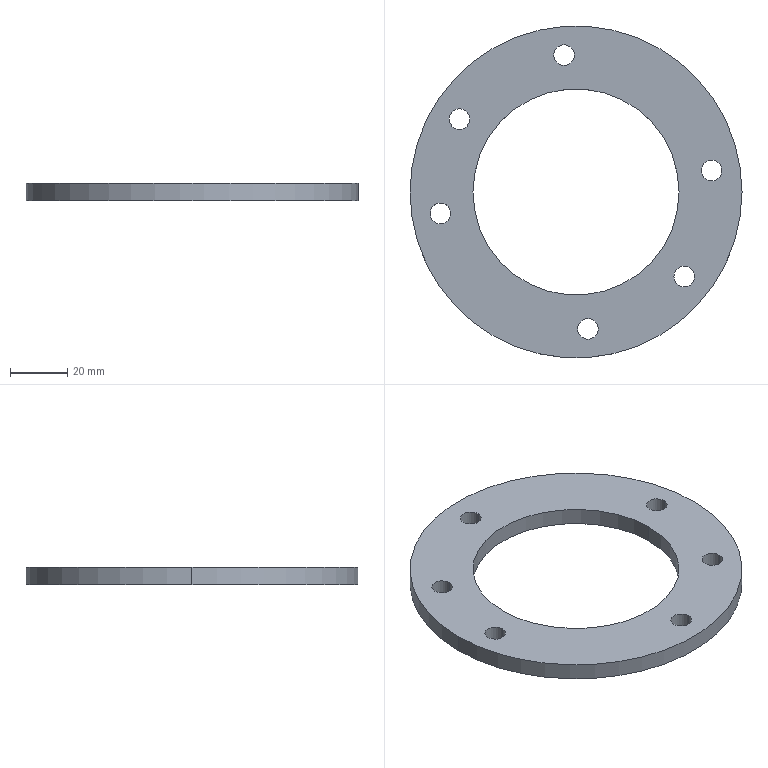Part | SolidWorks | features FlatPattern 1, SMBaseFlange 1, SheetMetal 1 | 1 solid | 18 faces | box 116 x 116 x 6 mm | volume 37515 mm3 | cylinder 16 | plane 2 | commonest cylinder face diameters 7.2 x12 72 x2 116 x2
STEP:
#1=CARTESIAN_POINT('',(-36.,0.,6.));
#2=VERTEX_POINT('',#1);
#3=CARTESIAN_POINT('',(36.,0.,6.));
#4=VERTEX_POINT('',#3);
#5=CARTESIAN_POINT('',(0.,0.,6.));
#6=DIRECTION('',(0.,0.,1.));
#7=DIRECTION('',(1.,0.,0.));
#8=AXIS2_PLACEMENT_3D('',#5,#6,#7);
#9=CIRCLE('',#8,36.);
#10=EDGE_CURVE('',#2,#4,#9,.T.);
#11=ORIENTED_EDGE('',*,*,#10,.T.);
#12=CARTESIAN_POINT('',(36.,0.,0.));
#13=VERTEX_POINT('',#12);
#14=CARTESIAN_POINT('',(36.,0.,6.));
#15=DIRECTION('',(0.,0.,-1.));
#16=VECTOR('',#15,1000.);
#17=LINE('',#14,#16);
#18=EDGE_CURVE('',#4,#13,#17,.T.);
#19=ORIENTED_EDGE('',*,*,#18,.T.);
#20=CARTESIAN_POINT('',(-36.,0.,0.));
#21=VERTEX_POINT('',#20);
#22=CARTESIAN_POINT('',(0.,0.,0.));
#23=DIRECTION('',(0.,0.,1.));
#24=DIRECTION('',(1.,0.,0.));
#25=AXIS2_PLACEMENT_3D('',#22,#23,#24);
#26=CIRCLE('',#25,36.);
#27=EDGE_CURVE('',#21,#13,#26,.T.);
#28=ORIENTED_EDGE('',*,*,#27,.F.);
#29=CARTESIAN_POINT('',(-36.,0.,6.));
#30=DIRECTION('',(0.,0.,-1.));
#31=VECTOR('',#30,1000.);
#32=LINE('',#29,#31);
#33=EDGE_CURVE('',#2,#21,#32,.T.);
#34=ORIENTED_EDGE('',*,*,#33,.F.);
#35=EDGE_LOOP('',(#11,#19,#28,#34));
#36=FACE_OUTER_BOUND('',#35,.T.);
#37=CARTESIAN_POINT('',(0.,0.,6.));
#38=DIRECTION('',(0.,0.,-1.));
#39=DIRECTION('',(-1.,0.,0.));
#40=AXIS2_PLACEMENT_3D('',#37,#38,#39);
#41=CYLINDRICAL_SURFACE('',#40,36.);
#42=ADVANCED_FACE('',(#36),#41,.F.);
#43=CARTESIAN_POINT('',(43.809,7.509,6.));
#44=VERTEX_POINT('',#43);
#45=CARTESIAN_POINT('',(51.009,7.509,6.));
#46=VERTEX_POINT('',#45);
#47=CARTESIAN_POINT('',(47.409,7.509,6.));
#48=DIRECTION('',(0.,0.,1.));
#49=DIRECTION('',(1.,0.,0.));
#50=AXIS2_PLACEMENT_3D('',#47,#48,#49);
#51=CIRCLE('',#50,3.6);
#52=EDGE_CURVE('',#44,#46,#51,.T.);
#53=ORIENTED_EDGE('',*,*,#52,.T.);
#54=CARTESIAN_POINT('',(51.009,7.509,0.));
#55=VERTEX_POINT('',#54);
#56=CARTESIAN_POINT('',(51.009,7.509,6.));
#57=DIRECTION('',(0.,0.,-1.));
#58=VECTOR('',#57,1000.);
#59=LINE('',#56,#58);
#60=EDGE_CURVE('',#46,#55,#59,.T.);
#61=ORIENTED_EDGE('',*,*,#60,.T.);
#62=CARTESIAN_POINT('',(43.809,7.509,0.));
#63=VERTEX_POINT('',#62);
#64=CARTESIAN_POINT('',(47.409,7.509,0.));
#65=DIRECTION('',(0.,0.,1.));
#66=DIRECTION('',(1.,0.,0.));
#67=AXIS2_PLACEMENT_3D('',#64,#65,#66);
#68=CIRCLE('',#67,3.6);
#69=EDGE_CURVE('',#63,#55,#68,.T.);
#70=ORIENTED_EDGE('',*,*,#69,.F.);
#71=CARTESIAN_POINT('',(43.809,7.509,6.));
#72=DIRECTION('',(0.,0.,-1.));
#73=VECTOR('',#72,1000.);
#74=LINE('',#71,#73);
#75=EDGE_CURVE('',#44,#63,#74,.T.);
#76=ORIENTED_EDGE('',*,*,#75,.F.);
#77=EDGE_LOOP('',(#53,#61,#70,#76));
#78=FACE_OUTER_BOUND('',#77,.T.);
#79=CARTESIAN_POINT('',(47.409,7.509,6.));
#80=DIRECTION('',(0.,0.,-1.));
#81=DIRECTION('',(-1.,0.,0.));
#82=AXIS2_PLACEMENT_3D('',#79,#80,#81);
#83=CYLINDRICAL_SURFACE('',#82,3.6);
#84=ADVANCED_FACE('',(#78),#83,.F.);
#85=CARTESIAN_POINT('',(34.225,-29.552,6.));
#86=VERTEX_POINT('',#85);
#87=CARTESIAN_POINT('',(41.425,-29.552,6.));
#88=VERTEX_POINT('',#87);
#89=CARTESIAN_POINT('',(37.825,-29.552,6.));
#90=DIRECTION('',(0.,0.,1.));
#91=DIRECTION('',(1.,0.,0.));
#92=AXIS2_PLACEMENT_3D('',#89,#90,#91);
#93=CIRCLE('',#92,3.6);
#94=EDGE_CURVE('',#86,#88,#93,.T.);
#95=ORIENTED_EDGE('',*,*,#94,.T.);
#96=CARTESIAN_POINT('',(41.425,-29.552,0.));
#97=VERTEX_POINT('',#96);
#98=CARTESIAN_POINT('',(41.425,-29.552,6.));
#99=DIRECTION('',(0.,0.,-1.));
#100=VECTOR('',#99,1000.);
#101=LINE('',#98,#100);
#102=EDGE_CURVE('',#88,#97,#101,.T.);
#103=ORIENTED_EDGE('',*,*,#102,.T.);
#104=CARTESIAN_POINT('',(34.225,-29.552,0.));
#105=VERTEX_POINT('',#104);
#106=CARTESIAN_POINT('',(37.825,-29.552,0.));
#107=DIRECTION('',(0.,0.,1.));
#108=DIRECTION('',(1.,0.,0.));
#109=AXIS2_PLACEMENT_3D('',#106,#107,#108);
#110=CIRCLE('',#109,3.6);
#111=EDGE_CURVE('',#105,#97,#110,.T.);
#112=ORIENTED_EDGE('',*,*,#111,.F.);
#113=CARTESIAN_POINT('',(34.225,-29.552,6.));
#114=DIRECTION('',(0.,0.,-1.));
#115=VECTOR('',#114,1000.);
#116=LINE('',#113,#115);
#117=EDGE_CURVE('',#86,#105,#116,.T.);
#118=ORIENTED_EDGE('',*,*,#117,.F.);
#119=EDGE_LOOP('',(#95,#103,#112,#118));
#120=FACE_OUTER_BOUND('',#119,.T.);
#121=CARTESIAN_POINT('',(37.825,-29.552,6.));
#122=DIRECTION('',(0.,0.,-1.));
#123=DIRECTION('',(-1.,0.,0.));
#124=AXIS2_PLACEMENT_3D('',#121,#122,#123);
#125=CYLINDRICAL_SURFACE('',#124,3.6);
#126=ADVANCED_FACE('',(#120),#125,.F.);
#127=CARTESIAN_POINT('',(0.5835,-47.817,6.));
#128=VERTEX_POINT('',#127);
#129=CARTESIAN_POINT('',(7.783,-47.817,6.));
#130=VERTEX_POINT('',#129);
#131=CARTESIAN_POINT('',(4.183,-47.817,6.));
#132=DIRECTION('',(0.,0.,1.));
#133=DIRECTION('',(1.,0.,0.));
#134=AXIS2_PLACEMENT_3D('',#131,#132,#133);
#135=CIRCLE('',#134,3.6);
#136=EDGE_CURVE('',#128,#130,#135,.T.);
#137=ORIENTED_EDGE('',*,*,#136,.T.);
#138=CARTESIAN_POINT('',(7.783,-47.817,0.));
#139=VERTEX_POINT('',#138);
#140=CARTESIAN_POINT('',(7.783,-47.817,6.));
#141=DIRECTION('',(0.,0.,-1.));
#142=VECTOR('',#141,1000.);
#143=LINE('',#140,#142);
#144=EDGE_CURVE('',#130,#139,#143,.T.);
#145=ORIENTED_EDGE('',*,*,#144,.T.);
#146=CARTESIAN_POINT('',(0.5835,-47.817,0.));
#147=VERTEX_POINT('',#146);
#148=CARTESIAN_POINT('',(4.183,-47.817,0.));
#149=DIRECTION('',(0.,0.,1.));
#150=DIRECTION('',(1.,0.,0.));
#151=AXIS2_PLACEMENT_3D('',#148,#149,#150);
#152=CIRCLE('',#151,3.6);
#153=EDGE_CURVE('',#147,#139,#152,.T.);
#154=ORIENTED_EDGE('',*,*,#153,.F.);
#155=CARTESIAN_POINT('',(0.5835,-47.817,6.));
#156=DIRECTION('',(0.,0.,-1.));
#157=VECTOR('',#156,1000.);
#158=LINE('',#155,#157);
#159=EDGE_CURVE('',#128,#147,#158,.T.);
#160=ORIENTED_EDGE('',*,*,#159,.F.);
#161=EDGE_LOOP('',(#137,#145,#154,#160));
#162=FACE_OUTER_BOUND('',#161,.T.);
#163=CARTESIAN_POINT('',(4.183,-47.817,6.));
#164=DIRECTION('',(0.,0.,-1.));
#165=DIRECTION('',(-1.,0.,0.));
#166=AXIS2_PLACEMENT_3D('',#163,#164,#165);
#167=CYLINDRICAL_SURFACE('',#166,3.6);
#168=ADVANCED_FACE('',(#162),#167,.F.);
#169=CARTESIAN_POINT('',(-51.009,-7.509,6.));
#170=VERTEX_POINT('',#169);
#171=CARTESIAN_POINT('',(-43.809,-7.509,6.));
#172=VERTEX_POINT('',#171);
#173=CARTESIAN_POINT('',(-47.409,-7.509,6.));
#174=DIRECTION('',(0.,0.,1.));
#175=DIRECTION('',(1.,0.,0.));
#176=AXIS2_PLACEMENT_3D('',#173,#174,#175);
#177=CIRCLE('',#176,3.6);
#178=EDGE_CURVE('',#170,#172,#177,.T.);
#179=ORIENTED_EDGE('',*,*,#178,.T.);
#180=CARTESIAN_POINT('',(-43.809,-7.509,0.));
#181=VERTEX_POINT('',#180);
#182=CARTESIAN_POINT('',(-43.809,-7.509,6.));
#183=DIRECTION('',(0.,0.,-1.));
#184=VECTOR('',#183,1000.);
#185=LINE('',#182,#184);
#186=EDGE_CURVE('',#172,#181,#185,.T.);
#187=ORIENTED_EDGE('',*,*,#186,.T.);
#188=CARTESIAN_POINT('',(-51.009,-7.509,0.));
#189=VERTEX_POINT('',#188);
#190=CARTESIAN_POINT('',(-47.409,-7.509,0.));
#191=DIRECTION('',(0.,0.,1.));
#192=DIRECTION('',(1.,0.,0.));
#193=AXIS2_PLACEMENT_3D('',#190,#191,#192);
#194=CIRCLE('',#193,3.6);
#195=EDGE_CURVE('',#189,#181,#194,.T.);
#196=ORIENTED_EDGE('',*,*,#195,.F.);
#197=CARTESIAN_POINT('',(-51.009,-7.509,6.));
#198=DIRECTION('',(0.,0.,-1.));
#199=VECTOR('',#198,1000.);
#200=LINE('',#197,#199);
#201=EDGE_CURVE('',#170,#189,#200,.T.);
#202=ORIENTED_EDGE('',*,*,#201,.F.);
#203=EDGE_LOOP('',(#179,#187,#196,#202));
#204=FACE_OUTER_BOUND('',#203,.T.);
#205=CARTESIAN_POINT('',(-47.409,-7.509,6.));
#206=DIRECTION('',(0.,0.,-1.));
#207=DIRECTION('',(-1.,0.,0.));
#208=AXIS2_PLACEMENT_3D('',#205,#206,#207);
#209=CYLINDRICAL_SURFACE('',#208,3.6);
#210=ADVANCED_FACE('',(#204),#209,.F.);
#211=CARTESIAN_POINT('',(-44.306,25.436,6.));
#212=VERTEX_POINT('',#211);
#213=CARTESIAN_POINT('',(-37.106,25.436,6.));
#214=VERTEX_POINT('',#213);
#215=CARTESIAN_POINT('',(-40.706,25.436,6.));
#216=DIRECTION('',(0.,0.,1.));
#217=DIRECTION('',(1.,0.,0.));
#218=AXIS2_PLACEMENT_3D('',#215,#216,#217);
#219=CIRCLE('',#218,3.6);
#220=EDGE_CURVE('',#212,#214,#219,.T.);
#221=ORIENTED_EDGE('',*,*,#220,.T.);
#222=CARTESIAN_POINT('',(-37.106,25.436,0.));
#223=VERTEX_POINT('',#222);
#224=CARTESIAN_POINT('',(-37.106,25.436,6.));
#225=DIRECTION('',(0.,0.,-1.));
#226=VECTOR('',#225,1000.);
#227=LINE('',#224,#226);
#228=EDGE_CURVE('',#214,#223,#227,.T.);
#229=ORIENTED_EDGE('',*,*,#228,.T.);
#230=CARTESIAN_POINT('',(-44.306,25.436,0.));
#231=VERTEX_POINT('',#230);
#232=CARTESIAN_POINT('',(-40.706,25.436,0.));
#233=DIRECTION('',(0.,0.,1.));
#234=DIRECTION('',(1.,0.,0.));
#235=AXIS2_PLACEMENT_3D('',#232,#233,#234);
#236=CIRCLE('',#235,3.6);
#237=EDGE_CURVE('',#231,#223,#236,.T.);
#238=ORIENTED_EDGE('',*,*,#237,.F.);
#239=CARTESIAN_POINT('',(-44.306,25.436,6.));
#240=DIRECTION('',(0.,0.,-1.));
#241=VECTOR('',#240,1000.);
#242=LINE('',#239,#241);
#243=EDGE_CURVE('',#212,#231,#242,.T.);
#244=ORIENTED_EDGE('',*,*,#243,.F.);
#245=EDGE_LOOP('',(#221,#229,#238,#244));
#246=FACE_OUTER_BOUND('',#245,.T.);
#247=CARTESIAN_POINT('',(-40.706,25.436,6.));
#248=DIRECTION('',(0.,0.,-1.));
#249=DIRECTION('',(-1.,0.,0.));
#250=AXIS2_PLACEMENT_3D('',#247,#248,#249);
#251=CYLINDRICAL_SURFACE('',#250,3.6);
#252=ADVANCED_FACE('',(#246),#251,.F.);
#253=CARTESIAN_POINT('',(-7.783,47.817,6.));
#254=VERTEX_POINT('',#253);
#255=CARTESIAN_POINT('',(-0.5835,47.817,6.));
#256=VERTEX_POINT('',#255);
#257=CARTESIAN_POINT('',(-4.183,47.817,6.));
#258=DIRECTION('',(0.,0.,1.));
#259=DIRECTION('',(1.,0.,0.));
#260=AXIS2_PLACEMENT_3D('',#257,#258,#259);
#261=CIRCLE('',#260,3.6);
#262=EDGE_CURVE('',#254,#256,#261,.T.);
#263=ORIENTED_EDGE('',*,*,#262,.T.);
#264=CARTESIAN_POINT('',(-0.5835,47.817,0.));
#265=VERTEX_POINT('',#264);
#266=CARTESIAN_POINT('',(-0.5835,47.817,6.));
#267=DIRECTION('',(0.,0.,-1.));
#268=VECTOR('',#267,1000.);
#269=LINE('',#266,#268);
#270=EDGE_CURVE('',#256,#265,#269,.T.);
#271=ORIENTED_EDGE('',*,*,#270,.T.);
#272=CARTESIAN_POINT('',(-7.783,47.817,0.));
#273=VERTEX_POINT('',#272);
#274=CARTESIAN_POINT('',(-4.183,47.817,0.));
#275=DIRECTION('',(0.,0.,1.));
#276=DIRECTION('',(1.,0.,0.));
#277=AXIS2_PLACEMENT_3D('',#274,#275,#276);
#278=CIRCLE('',#277,3.6);
#279=EDGE_CURVE('',#273,#265,#278,.T.);
#280=ORIENTED_EDGE('',*,*,#279,.F.);
#281=CARTESIAN_POINT('',(-7.783,47.817,6.));
#282=DIRECTION('',(0.,0.,-1.));
#283=VECTOR('',#282,1000.);
#284=LINE('',#281,#283);
#285=EDGE_CURVE('',#254,#273,#284,.T.);
#286=ORIENTED_EDGE('',*,*,#285,.F.);
#287=EDGE_LOOP('',(#263,#271,#280,#286));
#288=FACE_OUTER_BOUND('',#287,.T.);
#289=CARTESIAN_POINT('',(-4.183,47.817,6.));
#290=DIRECTION('',(0.,0.,-1.));
#291=DIRECTION('',(-1.,0.,0.));
#292=AXIS2_PLACEMENT_3D('',#289,#290,#291);
#293=CYLINDRICAL_SURFACE('',#292,3.6);
#294=ADVANCED_FACE('',(#288),#293,.F.);
#295=CARTESIAN_POINT('',(58.,0.,6.));
#296=VERTEX_POINT('',#295);
#297=CARTESIAN_POINT('',(-58.,0.,6.));
#298=VERTEX_POINT('',#297);
#299=CARTESIAN_POINT('',(0.,0.,6.));
#300=DIRECTION('',(0.,0.,1.));
#301=DIRECTION('',(1.,0.,0.));
#302=AXIS2_PLACEMENT_3D('',#299,#300,#301);
#303=CIRCLE('',#302,58.);
#304=EDGE_CURVE('',#296,#298,#303,.T.);
#305=ORIENTED_EDGE('',*,*,#304,.F.);
#306=CARTESIAN_POINT('',(58.,0.,0.));
#307=VERTEX_POINT('',#306);
#308=CARTESIAN_POINT('',(58.,0.,6.));
#309=DIRECTION('',(0.,0.,-1.));
#310=VECTOR('',#309,1000.);
#311=LINE('',#308,#310);
#312=EDGE_CURVE('',#296,#307,#311,.T.);
#313=ORIENTED_EDGE('',*,*,#312,.T.);
#314=CARTESIAN_POINT('',(-58.,0.,0.));
#315=VERTEX_POINT('',#314);
#316=CARTESIAN_POINT('',(0.,0.,0.));
#317=DIRECTION('',(0.,0.,1.));
#318=DIRECTION('',(1.,0.,0.));
#319=AXIS2_PLACEMENT_3D('',#316,#317,#318);
#320=CIRCLE('',#319,58.);
#321=EDGE_CURVE('',#307,#315,#320,.T.);
#322=ORIENTED_EDGE('',*,*,#321,.T.);
#323=CARTESIAN_POINT('',(-58.,0.,6.));
#324=DIRECTION('',(0.,0.,-1.));
#325=VECTOR('',#324,1000.);
#326=LINE('',#323,#325);
#327=EDGE_CURVE('',#298,#315,#326,.T.);
#328=ORIENTED_EDGE('',*,*,#327,.F.);
#329=EDGE_LOOP('',(#305,#313,#322,#328));
#330=FACE_OUTER_BOUND('',#329,.T.);
#331=CARTESIAN_POINT('',(0.,0.,6.));
#332=DIRECTION('',(0.,0.,-1.));
#333=DIRECTION('',(-1.,0.,0.));
#334=AXIS2_PLACEMENT_3D('',#331,#332,#333);
#335=CYLINDRICAL_SURFACE('',#334,58.);
#336=ADVANCED_FACE('',(#330),#335,.T.);
#337=ORIENTED_EDGE('',*,*,#52,.F.);
#338=CARTESIAN_POINT('',(47.409,7.509,6.));
#339=DIRECTION('',(0.,0.,1.));
#340=DIRECTION('',(1.,0.,0.));
#341=AXIS2_PLACEMENT_3D('',#338,#339,#340);
#342=CIRCLE('',#341,3.6);
#343=EDGE_CURVE('',#46,#44,#342,.T.);
#344=ORIENTED_EDGE('',*,*,#343,.F.);
#345=EDGE_LOOP('',(#337,#344));
#346=FACE_BOUND('',#345,.T.);
#347=ORIENTED_EDGE('',*,*,#136,.F.);
#348=CARTESIAN_POINT('',(4.183,-47.817,6.));
#349=DIRECTION('',(0.,0.,1.));
#350=DIRECTION('',(1.,0.,0.));
#351=AXIS2_PLACEMENT_3D('',#348,#349,#350);
#352=CIRCLE('',#351,3.6);
#353=EDGE_CURVE('',#130,#128,#352,.T.);
#354=ORIENTED_EDGE('',*,*,#353,.F.);
#355=EDGE_LOOP('',(#347,#354));
#356=FACE_BOUND('',#355,.T.);
#357=ORIENTED_EDGE('',*,*,#220,.F.);
#358=CARTESIAN_POINT('',(-40.706,25.436,6.));
#359=DIRECTION('',(0.,0.,1.));
#360=DIRECTION('',(1.,0.,0.));
#361=AXIS2_PLACEMENT_3D('',#358,#359,#360);
#362=CIRCLE('',#361,3.6);
#363=EDGE_CURVE('',#214,#212,#362,.T.);
#364=ORIENTED_EDGE('',*,*,#363,.F.);
#365=EDGE_LOOP('',(#357,#364));
#366=FACE_BOUND('',#365,.T.);
#367=CARTESIAN_POINT('',(0.,0.,6.));
#368=DIRECTION('',(0.,0.,1.));
#369=DIRECTION('',(1.,0.,0.));
#370=AXIS2_PLACEMENT_3D('',#367,#368,#369);
#371=CIRCLE('',#370,58.);
#372=EDGE_CURVE('',#298,#296,#371,.T.);
#373=ORIENTED_EDGE('',*,*,#372,.T.);
#374=ORIENTED_EDGE('',*,*,#304,.T.);
#375=EDGE_LOOP('',(#373,#374));
#376=FACE_OUTER_BOUND('',#375,.T.);
#377=ORIENTED_EDGE('',*,*,#262,.F.);
#378=CARTESIAN_POINT('',(-4.183,47.817,6.));
#379=DIRECTION('',(0.,0.,1.));
#380=DIRECTION('',(1.,0.,0.));
#381=AXIS2_PLACEMENT_3D('',#378,#379,#380);
#382=CIRCLE('',#381,3.6);
#383=EDGE_CURVE('',#256,#254,#382,.T.);
#384=ORIENTED_EDGE('',*,*,#383,.F.);
#385=EDGE_LOOP('',(#377,#384));
#386=FACE_BOUND('',#385,.T.);
#387=ORIENTED_EDGE('',*,*,#178,.F.);
#388=CARTESIAN_POINT('',(-47.409,-7.509,6.));
#389=DIRECTION('',(0.,0.,1.));
#390=DIRECTION('',(1.,0.,0.));
#391=AXIS2_PLACEMENT_3D('',#388,#389,#390);
#392=CIRCLE('',#391,3.6);
#393=EDGE_CURVE('',#172,#170,#392,.T.);
#394=ORIENTED_EDGE('',*,*,#393,.F.);
#395=EDGE_LOOP('',(#387,#394));
#396=FACE_BOUND('',#395,.T.);
#397=ORIENTED_EDGE('',*,*,#94,.F.);
#398=CARTESIAN_POINT('',(37.825,-29.552,6.));
#399=DIRECTION('',(0.,0.,1.));
#400=DIRECTION('',(1.,0.,0.));
#401=AXIS2_PLACEMENT_3D('',#398,#399,#400);
#402=CIRCLE('',#401,3.6);
#403=EDGE_CURVE('',#88,#86,#402,.T.);
#404=ORIENTED_EDGE('',*,*,#403,.F.);
#405=EDGE_LOOP('',(#397,#404));
#406=FACE_BOUND('',#405,.T.);
#407=ORIENTED_EDGE('',*,*,#10,.F.);
#408=CARTESIAN_POINT('',(0.,0.,6.));
#409=DIRECTION('',(0.,0.,1.));
#410=DIRECTION('',(1.,0.,0.));
#411=AXIS2_PLACEMENT_3D('',#408,#409,#410);
#412=CIRCLE('',#411,36.);
#413=EDGE_CURVE('',#4,#2,#412,.T.);
#414=ORIENTED_EDGE('',*,*,#413,.F.);
#415=EDGE_LOOP('',(#407,#414));
#416=FACE_BOUND('',#415,.T.);
#417=CARTESIAN_POINT('',(0.,0.,6.));
#418=DIRECTION('',(0.,0.,1.));
#419=DIRECTION('',(1.,0.,0.));
#420=AXIS2_PLACEMENT_3D('',#417,#418,#419);
#421=PLANE('',#420);
#422=ADVANCED_FACE('',(#346,#356,#366,#376,#386,#396,#406,#416),#421,.T.);
#423=CARTESIAN_POINT('',(0.,0.,0.));
#424=DIRECTION('',(0.,0.,1.));
#425=DIRECTION('',(1.,0.,0.));
#426=AXIS2_PLACEMENT_3D('',#423,#424,#425);
#427=CIRCLE('',#426,58.);
#428=EDGE_CURVE('',#315,#307,#427,.T.);
#429=ORIENTED_EDGE('',*,*,#428,.F.);
#430=ORIENTED_EDGE('',*,*,#321,.F.);
#431=EDGE_LOOP('',(#429,#430));
#432=FACE_OUTER_BOUND('',#431,.T.);
#433=ORIENTED_EDGE('',*,*,#279,.T.);
#434=CARTESIAN_POINT('',(-4.183,47.817,0.));
#435=DIRECTION('',(0.,0.,1.));
#436=DIRECTION('',(1.,0.,0.));
#437=AXIS2_PLACEMENT_3D('',#434,#435,#436);
#438=CIRCLE('',#437,3.6);
#439=EDGE_CURVE('',#265,#273,#438,.T.);
#440=ORIENTED_EDGE('',*,*,#439,.T.);
#441=EDGE_LOOP('',(#433,#440));
#442=FACE_BOUND('',#441,.T.);
#443=ORIENTED_EDGE('',*,*,#237,.T.);
#444=CARTESIAN_POINT('',(-40.706,25.436,0.));
#445=DIRECTION('',(0.,0.,1.));
#446=DIRECTION('',(1.,0.,0.));
#447=AXIS2_PLACEMENT_3D('',#444,#445,#446);
#448=CIRCLE('',#447,3.6);
#449=EDGE_CURVE('',#223,#231,#448,.T.);
#450=ORIENTED_EDGE('',*,*,#449,.T.);
#451=EDGE_LOOP('',(#443,#450));
#452=FACE_BOUND('',#451,.T.);
#453=ORIENTED_EDGE('',*,*,#195,.T.);
#454=CARTESIAN_POINT('',(-47.409,-7.509,0.));
#455=DIRECTION('',(0.,0.,1.));
#456=DIRECTION('',(1.,0.,0.));
#457=AXIS2_PLACEMENT_3D('',#454,#455,#456);
#458=CIRCLE('',#457,3.6);
#459=EDGE_CURVE('',#181,#189,#458,.T.);
#460=ORIENTED_EDGE('',*,*,#459,.T.);
#461=EDGE_LOOP('',(#453,#460));
#462=FACE_BOUND('',#461,.T.);
#463=ORIENTED_EDGE('',*,*,#153,.T.);
#464=CARTESIAN_POINT('',(4.183,-47.817,0.));
#465=DIRECTION('',(0.,0.,1.));
#466=DIRECTION('',(1.,0.,0.));
#467=AXIS2_PLACEMENT_3D('',#464,#465,#466);
#468=CIRCLE('',#467,3.6);
#469=EDGE_CURVE('',#139,#147,#468,.T.);
#470=ORIENTED_EDGE('',*,*,#469,.T.);
#471=EDGE_LOOP('',(#463,#470));
#472=FACE_BOUND('',#471,.T.);
#473=ORIENTED_EDGE('',*,*,#111,.T.);
#474=CARTESIAN_POINT('',(37.825,-29.552,0.));
#475=DIRECTION('',(0.,0.,1.));
#476=DIRECTION('',(1.,0.,0.));
#477=AXIS2_PLACEMENT_3D('',#474,#475,#476);
#478=CIRCLE('',#477,3.6);
#479=EDGE_CURVE('',#97,#105,#478,.T.);
#480=ORIENTED_EDGE('',*,*,#479,.T.);
#481=EDGE_LOOP('',(#473,#480));
#482=FACE_BOUND('',#481,.T.);
#483=ORIENTED_EDGE('',*,*,#69,.T.);
#484=CARTESIAN_POINT('',(47.409,7.509,0.));
#485=DIRECTION('',(0.,0.,1.));
#486=DIRECTION('',(1.,0.,0.));
#487=AXIS2_PLACEMENT_3D('',#484,#485,#486);
#488=CIRCLE('',#487,3.6);
#489=EDGE_CURVE('',#55,#63,#488,.T.);
#490=ORIENTED_EDGE('',*,*,#489,.T.);
#491=EDGE_LOOP('',(#483,#490));
#492=FACE_BOUND('',#491,.T.);
#493=ORIENTED_EDGE('',*,*,#27,.T.);
#494=CARTESIAN_POINT('',(0.,0.,0.));
#495=DIRECTION('',(0.,0.,1.));
#496=DIRECTION('',(1.,0.,0.));
#497=AXIS2_PLACEMENT_3D('',#494,#495,#496);
#498=CIRCLE('',#497,36.);
#499=EDGE_CURVE('',#13,#21,#498,.T.);
#500=ORIENTED_EDGE('',*,*,#499,.T.);
#501=EDGE_LOOP('',(#493,#500));
#502=FACE_BOUND('',#501,.T.);
#503=CARTESIAN_POINT('',(0.,0.,0.));
#504=DIRECTION('',(0.,0.,1.));
#505=DIRECTION('',(1.,0.,0.));
#506=AXIS2_PLACEMENT_3D('',#503,#504,#505);
#507=PLANE('',#506);
#508=ADVANCED_FACE('',(#432,#442,#452,#462,#472,#482,#492,#502),#507,.F.);
#509=ORIENTED_EDGE('',*,*,#312,.F.);
#510=ORIENTED_EDGE('',*,*,#372,.F.);
#511=ORIENTED_EDGE('',*,*,#327,.T.);
#512=ORIENTED_EDGE('',*,*,#428,.T.);
#513=EDGE_LOOP('',(#509,#510,#511,#512));
#514=FACE_OUTER_BOUND('',#513,.T.);
#515=CARTESIAN_POINT('',(0.,0.,6.));
#516=DIRECTION('',(0.,0.,-1.));
#517=DIRECTION('',(-1.,0.,0.));
#518=AXIS2_PLACEMENT_3D('',#515,#516,#517);
#519=CYLINDRICAL_SURFACE('',#518,58.);
#520=ADVANCED_FACE('',(#514),#519,.T.);
#521=ORIENTED_EDGE('',*,*,#270,.F.);
#522=ORIENTED_EDGE('',*,*,#383,.T.);
#523=ORIENTED_EDGE('',*,*,#285,.T.);
#524=ORIENTED_EDGE('',*,*,#439,.F.);
#525=EDGE_LOOP('',(#521,#522,#523,#524));
#526=FACE_OUTER_BOUND('',#525,.T.);
#527=CARTESIAN_POINT('',(-4.183,47.817,6.));
#528=DIRECTION('',(0.,0.,-1.));
#529=DIRECTION('',(-1.,0.,0.));
#530=AXIS2_PLACEMENT_3D('',#527,#528,#529);
#531=CYLINDRICAL_SURFACE('',#530,3.6);
#532=ADVANCED_FACE('',(#526),#531,.F.);
#533=ORIENTED_EDGE('',*,*,#228,.F.);
#534=ORIENTED_EDGE('',*,*,#363,.T.);
#535=ORIENTED_EDGE('',*,*,#243,.T.);
#536=ORIENTED_EDGE('',*,*,#449,.F.);
#537=EDGE_LOOP('',(#533,#534,#535,#536));
#538=FACE_OUTER_BOUND('',#537,.T.);
#539=CARTESIAN_POINT('',(-40.706,25.436,6.));
#540=DIRECTION('',(0.,0.,-1.));
#541=DIRECTION('',(-1.,0.,0.));
#542=AXIS2_PLACEMENT_3D('',#539,#540,#541);
#543=CYLINDRICAL_SURFACE('',#542,3.6);
#544=ADVANCED_FACE('',(#538),#543,.F.);
#545=ORIENTED_EDGE('',*,*,#186,.F.);
#546=ORIENTED_EDGE('',*,*,#393,.T.);
#547=ORIENTED_EDGE('',*,*,#201,.T.);
#548=ORIENTED_EDGE('',*,*,#459,.F.);
#549=EDGE_LOOP('',(#545,#546,#547,#548));
#550=FACE_OUTER_BOUND('',#549,.T.);
#551=CARTESIAN_POINT('',(-47.409,-7.509,6.));
#552=DIRECTION('',(0.,0.,-1.));
#553=DIRECTION('',(-1.,0.,0.));
#554=AXIS2_PLACEMENT_3D('',#551,#552,#553);
#555=CYLINDRICAL_SURFACE('',#554,3.6);
#556=ADVANCED_FACE('',(#550),#555,.F.);
#557=ORIENTED_EDGE('',*,*,#144,.F.);
#558=ORIENTED_EDGE('',*,*,#353,.T.);
#559=ORIENTED_EDGE('',*,*,#159,.T.);
#560=ORIENTED_EDGE('',*,*,#469,.F.);
#561=EDGE_LOOP('',(#557,#558,#559,#560));
#562=FACE_OUTER_BOUND('',#561,.T.);
#563=CARTESIAN_POINT('',(4.183,-47.817,6.));
#564=DIRECTION('',(0.,0.,-1.));
#565=DIRECTION('',(-1.,0.,0.));
#566=AXIS2_PLACEMENT_3D('',#563,#564,#565);
#567=CYLINDRICAL_SURFACE('',#566,3.6);
#568=ADVANCED_FACE('',(#562),#567,.F.);
#569=ORIENTED_EDGE('',*,*,#102,.F.);
#570=ORIENTED_EDGE('',*,*,#403,.T.);
#571=ORIENTED_EDGE('',*,*,#117,.T.);
#572=ORIENTED_EDGE('',*,*,#479,.F.);
#573=EDGE_LOOP('',(#569,#570,#571,#572));
#574=FACE_OUTER_BOUND('',#573,.T.);
#575=CARTESIAN_POINT('',(37.825,-29.552,6.));
#576=DIRECTION('',(0.,0.,-1.));
#577=DIRECTION('',(-1.,0.,0.));
#578=AXIS2_PLACEMENT_3D('',#575,#576,#577);
#579=CYLINDRICAL_SURFACE('',#578,3.6);
#580=ADVANCED_FACE('',(#574),#579,.F.);
#581=ORIENTED_EDGE('',*,*,#60,.F.);
#582=ORIENTED_EDGE('',*,*,#343,.T.);
#583=ORIENTED_EDGE('',*,*,#75,.T.);
#584=ORIENTED_EDGE('',*,*,#489,.F.);
#585=EDGE_LOOP('',(#581,#582,#583,#584));
#586=FACE_OUTER_BOUND('',#585,.T.);
#587=CARTESIAN_POINT('',(47.409,7.509,6.));
#588=DIRECTION('',(0.,0.,-1.));
#589=DIRECTION('',(-1.,0.,0.));
#590=AXIS2_PLACEMENT_3D('',#587,#588,#589);
#591=CYLINDRICAL_SURFACE('',#590,3.6);
#592=ADVANCED_FACE('',(#586),#591,.F.);
#593=ORIENTED_EDGE('',*,*,#18,.F.);
#594=ORIENTED_EDGE('',*,*,#413,.T.);
#595=ORIENTED_EDGE('',*,*,#33,.T.);
#596=ORIENTED_EDGE('',*,*,#499,.F.);
#597=EDGE_LOOP('',(#593,#594,#595,#596));
#598=FACE_OUTER_BOUND('',#597,.T.);
#599=CARTESIAN_POINT('',(0.,0.,6.));
#600=DIRECTION('',(0.,0.,-1.));
#601=DIRECTION('',(-1.,0.,0.));
#602=AXIS2_PLACEMENT_3D('',#599,#600,#601);
#603=CYLINDRICAL_SURFACE('',#602,36.);
#604=ADVANCED_FACE('',(#598),#603,.F.);
#605=CLOSED_SHELL('',(#42,#84,#126,#168,#210,#252,#294,#336,#422,#508,#520,#532,#544,#556,#568,#580,#592,#604));
#606=MANIFOLD_SOLID_BREP('',#605);
#607=CARTESIAN_POINT('',(0.,0.,0.));
#608=DIRECTION('',(0.,0.,1.));
#609=DIRECTION('',(1.,0.,0.));
#610=AXIS2_PLACEMENT_3D('',#607,#608,#609);
#611=(LENGTH_UNIT()NAMED_UNIT(*)SI_UNIT(.MILLI.,.METRE.));
#612=UNCERTAINTY_MEASURE_WITH_UNIT(LENGTH_MEASURE(0.00001),#611,'','');
#613=(NAMED_UNIT(*)PLANE_ANGLE_UNIT()SI_UNIT($,.RADIAN.));
#614=(NAMED_UNIT(*)SI_UNIT($,.STERADIAN.)SOLID_ANGLE_UNIT());
#615=(GEOMETRIC_REPRESENTATION_CONTEXT(3)GLOBAL_UNCERTAINTY_ASSIGNED_CONTEXT((#612))GLOBAL_UNIT_ASSIGNED_CONTEXT((#611,#613,#614))REPRESENTATION_CONTEXT('',''));
#616=ADVANCED_BREP_SHAPE_REPRESENTATION('',(#606,#610),#615);